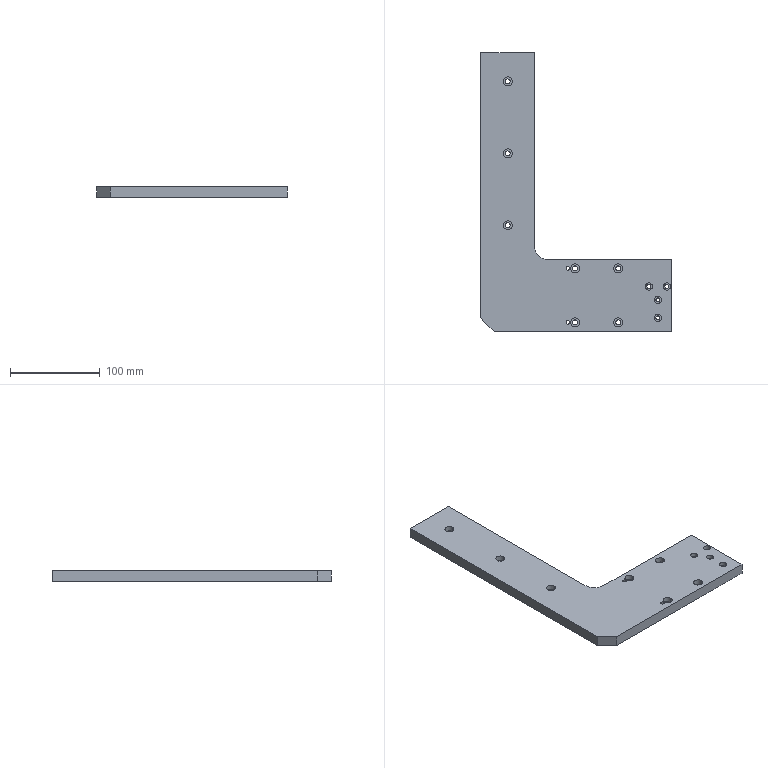Part | STEP file | 2069 Support plate B | 1 solid | 77 faces | box 212 x 310 x 12 mm | volume 361905 mm3 | cylinder 53 | plane 20 | cone 4 | commonest cylinder face diameters 5.5 x14 10 x14 4.5 x8 8 x8 4 x4 4.2 x4